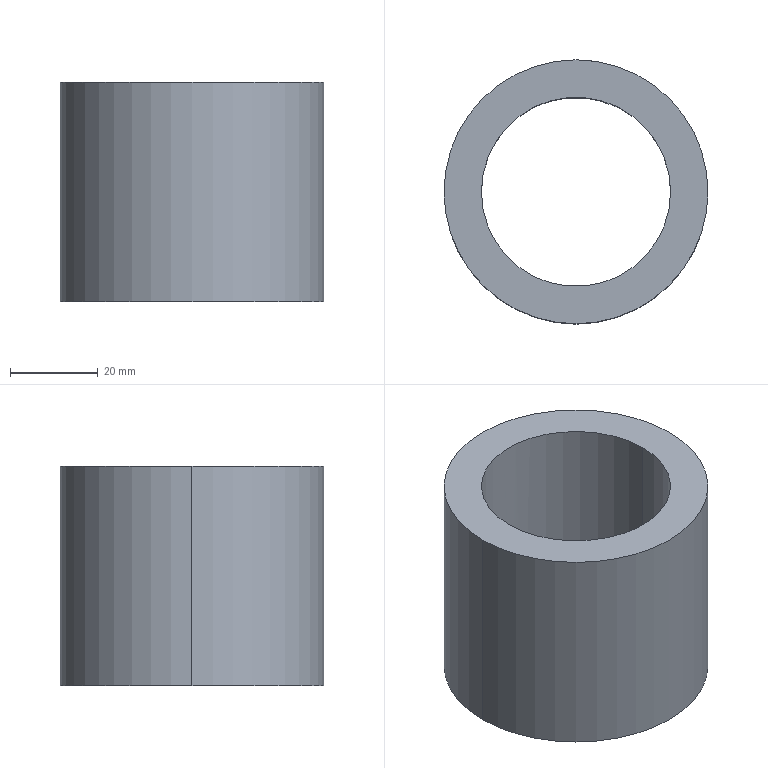Part | SolidWorks | features 3DProfileFeature 1, Cut 1, Extrusion 1, HoleWzd 1, ICE 1 | 1 solid | 8 faces | box 60 x 60 x 50 mm | volume 68595 mm3 | cylinder 6 | plane 2 | commonest cylinder face diameters 5 x2 43 x2 60 x2
STEP:
#1=CARTESIAN_POINT('',(4.954,20.921,-40.));
#2=VERTEX_POINT('',#1);
#3=CARTESIAN_POINT('',(-0.01248,21.5,-40.));
#4=VERTEX_POINT('',#3);
#5=CARTESIAN_POINT('',(4.954,20.921,-40.));
#6=CARTESIAN_POINT('',(4.954,20.921,-40.163));
#7=CARTESIAN_POINT('',(4.938,20.925,-40.325));
#8=CARTESIAN_POINT('',(4.876,20.94,-40.648));
#9=CARTESIAN_POINT('',(4.829,20.951,-40.806));
#10=CARTESIAN_POINT('',(4.706,20.979,-41.107));
#11=CARTESIAN_POINT('',(4.63,20.996,-41.252));
#12=CARTESIAN_POINT('',(4.451,21.034,-41.525));
#13=CARTESIAN_POINT('',(4.35,21.056,-41.651));
#14=CARTESIAN_POINT('',(4.123,21.101,-41.882));
#15=CARTESIAN_POINT('',(3.996,21.126,-41.987));
#16=CARTESIAN_POINT('',(3.729,21.175,-42.169));
#17=CARTESIAN_POINT('',(3.587,21.199,-42.246));
#18=CARTESIAN_POINT('',(3.288,21.248,-42.372));
#19=CARTESIAN_POINT('',(3.131,21.271,-42.42));
#20=CARTESIAN_POINT('',(2.815,21.316,-42.484));
#21=CARTESIAN_POINT('',(2.654,21.336,-42.5));
#22=CARTESIAN_POINT('',(2.325,21.375,-42.5));
#23=CARTESIAN_POINT('',(2.164,21.391,-42.484));
#24=CARTESIAN_POINT('',(1.845,21.421,-42.421));
#25=CARTESIAN_POINT('',(1.687,21.434,-42.373));
#26=CARTESIAN_POINT('',(1.384,21.456,-42.247));
#27=CARTESIAN_POINT('',(1.241,21.465,-42.171));
#28=CARTESIAN_POINT('',(0.9689,21.479,-41.989));
#29=CARTESIAN_POINT('',(0.8401,21.484,-41.884));
#30=CARTESIAN_POINT('',(0.6089,21.492,-41.654));
#31=CARTESIAN_POINT('',(0.505,21.494,-41.528));
#32=CARTESIAN_POINT('',(0.3212,21.498,-41.255));
#33=CARTESIAN_POINT('',(0.2431,21.499,-41.11));
#34=CARTESIAN_POINT('',(0.05455,21.5,-40.659));
#35=CARTESIAN_POINT('',(-0.01248,21.5,-40.331));
#36=CARTESIAN_POINT('',(-0.01248,21.5,-40.));
#37=B_SPLINE_CURVE_WITH_KNOTS('',3,(#5,#6,#7,#8,#9,#10,#11,#12,#13,#14,#15,#16,#17,#18,#19,#20,#21,#22,#23,#24,#25,#26,#27,#28,#29,#30,#31,#32,#33,#34,#35,#36),.UNSPECIFIED.,.F.,.F.,(4,2,2,2,2,2,2,2,2,2,2,2,2,2,2,4),(0.007823,0.008312,0.0088,0.009289,0.009778,0.01027,0.01076,0.01124,0.01173,0.01222,0.01271,0.0132,0.01369,0.01418,0.01467,0.01564),.UNSPECIFIED.);
#38=EDGE_CURVE('',#2,#4,#37,.T.);
#39=ORIENTED_EDGE('',*,*,#38,.F.);
#40=CARTESIAN_POINT('',(5.942,29.406,-40.));
#41=VERTEX_POINT('',#40);
#42=CARTESIAN_POINT('',(5.954,29.509,-40.));
#43=DIRECTION('',(0.1157,0.9933,0.));
#44=VECTOR('',#43,1000.);
#45=LINE('',#42,#44);
#46=EDGE_CURVE('',#2,#41,#45,.T.);
#47=ORIENTED_EDGE('',*,*,#46,.T.);
#48=CARTESIAN_POINT('',(0.9758,29.984,-40.));
#49=VERTEX_POINT('',#48);
#50=CARTESIAN_POINT('',(5.942,29.406,-40.));
#51=CARTESIAN_POINT('',(5.942,29.406,-40.163));
#52=CARTESIAN_POINT('',(5.927,29.409,-40.325));
#53=CARTESIAN_POINT('',(5.864,29.421,-40.648));
#54=CARTESIAN_POINT('',(5.816,29.431,-40.806));
#55=CARTESIAN_POINT('',(5.694,29.455,-41.107));
#56=CARTESIAN_POINT('',(5.618,29.469,-41.252));
#57=CARTESIAN_POINT('',(5.438,29.503,-41.525));
#58=CARTESIAN_POINT('',(5.336,29.522,-41.651));
#59=CARTESIAN_POINT('',(5.109,29.562,-41.882));
#60=CARTESIAN_POINT('',(4.982,29.584,-41.987));
#61=CARTESIAN_POINT('',(4.713,29.628,-42.169));
#62=CARTESIAN_POINT('',(4.572,29.65,-42.246));
#63=CARTESIAN_POINT('',(4.272,29.695,-42.372));
#64=CARTESIAN_POINT('',(4.115,29.717,-42.42));
#65=CARTESIAN_POINT('',(3.798,29.759,-42.484));
#66=CARTESIAN_POINT('',(3.637,29.779,-42.5));
#67=CARTESIAN_POINT('',(3.309,29.817,-42.5));
#68=CARTESIAN_POINT('',(3.147,29.835,-42.484));
#69=CARTESIAN_POINT('',(2.829,29.867,-42.421));
#70=CARTESIAN_POINT('',(2.671,29.881,-42.373));
#71=CARTESIAN_POINT('',(2.369,29.907,-42.247));
#72=CARTESIAN_POINT('',(2.226,29.918,-42.171));
#73=CARTESIAN_POINT('',(1.954,29.937,-41.99));
#74=CARTESIAN_POINT('',(1.826,29.945,-41.884));
#75=CARTESIAN_POINT('',(1.595,29.958,-41.654));
#76=CARTESIAN_POINT('',(1.491,29.963,-41.528));
#77=CARTESIAN_POINT('',(1.308,29.972,-41.255));
#78=CARTESIAN_POINT('',(1.23,29.975,-41.11));
#79=CARTESIAN_POINT('',(1.042,29.982,-40.659));
#80=CARTESIAN_POINT('',(0.9758,29.984,-40.33));
#81=CARTESIAN_POINT('',(0.9758,29.984,-40.));
#82=B_SPLINE_CURVE_WITH_KNOTS('',3,(#50,#51,#52,#53,#54,#55,#56,#57,#58,#59,#60,#61,#62,#63,#64,#65,#66,#67,#68,#69,#70,#71,#72,#73,#74,#75,#76,#77,#78,#79,#80,#81),.UNSPECIFIED.,.F.,.F.,(4,2,2,2,2,2,2,2,2,2,2,2,2,2,2,4),(0.00782,0.008308,0.008797,0.009285,0.009774,0.01026,0.01075,0.01124,0.01173,0.01222,0.01271,0.01319,0.01368,0.01417,0.01466,0.01564),.UNSPECIFIED.);
#83=EDGE_CURVE('',#41,#49,#82,.T.);
#84=ORIENTED_EDGE('',*,*,#83,.T.);
#85=CARTESIAN_POINT('',(0.9879,30.088,-40.));
#86=DIRECTION('',(0.1157,0.9933,0.));
#87=VECTOR('',#86,1000.);
#88=LINE('',#85,#87);
#89=EDGE_CURVE('',#4,#49,#88,.T.);
#90=ORIENTED_EDGE('',*,*,#89,.F.);
#91=EDGE_LOOP('',(#39,#47,#84,#90));
#92=FACE_OUTER_BOUND('',#91,.T.);
#93=CARTESIAN_POINT('',(3.471,29.799,-40.));
#94=DIRECTION('',(0.1157,0.9933,0.));
#95=DIRECTION('',(-0.9933,0.1157,0.));
#96=AXIS2_PLACEMENT_3D('',#93,#94,#95);
#97=CYLINDRICAL_SURFACE('',#96,2.5);
#98=ADVANCED_FACE('',(#92),#97,.F.);
#99=CARTESIAN_POINT('',(0.9758,29.984,-40.));
#100=CARTESIAN_POINT('',(0.9758,29.984,-39.835));
#101=CARTESIAN_POINT('',(0.9921,29.984,-39.672));
#102=CARTESIAN_POINT('',(1.056,29.981,-39.353));
#103=CARTESIAN_POINT('',(1.104,29.98,-39.194));
#104=CARTESIAN_POINT('',(1.23,29.975,-38.891));
#105=CARTESIAN_POINT('',(1.307,29.972,-38.747));
#106=CARTESIAN_POINT('',(1.489,29.963,-38.476));
#107=CARTESIAN_POINT('',(1.594,29.958,-38.347));
#108=CARTESIAN_POINT('',(1.825,29.945,-38.117));
#109=CARTESIAN_POINT('',(1.951,29.937,-38.013));
#110=CARTESIAN_POINT('',(2.223,29.918,-37.83));
#111=CARTESIAN_POINT('',(2.369,29.907,-37.753));
#112=CARTESIAN_POINT('',(2.669,29.881,-37.628));
#113=CARTESIAN_POINT('',(2.826,29.867,-37.58));
#114=CARTESIAN_POINT('',(3.147,29.835,-37.516));
#115=CARTESIAN_POINT('',(3.308,29.817,-37.5));
#116=CARTESIAN_POINT('',(3.632,29.78,-37.5));
#117=CARTESIAN_POINT('',(3.797,29.759,-37.516));
#118=CARTESIAN_POINT('',(4.115,29.717,-37.58));
#119=CARTESIAN_POINT('',(4.269,29.695,-37.627));
#120=CARTESIAN_POINT('',(4.569,29.65,-37.753));
#121=CARTESIAN_POINT('',(4.713,29.628,-37.831));
#122=CARTESIAN_POINT('',(4.981,29.584,-38.012));
#123=CARTESIAN_POINT('',(5.105,29.563,-38.115));
#124=CARTESIAN_POINT('',(5.336,29.522,-38.349));
#125=CARTESIAN_POINT('',(5.438,29.503,-38.475));
#126=CARTESIAN_POINT('',(5.616,29.47,-38.746));
#127=CARTESIAN_POINT('',(5.693,29.455,-38.892));
#128=CARTESIAN_POINT('',(5.817,29.431,-39.195));
#129=CARTESIAN_POINT('',(5.863,29.421,-39.351));
#130=CARTESIAN_POINT('',(5.926,29.409,-39.671));
#131=CARTESIAN_POINT('',(5.942,29.406,-39.837));
#132=CARTESIAN_POINT('',(5.942,29.406,-40.));
#133=B_SPLINE_CURVE_WITH_KNOTS('',3,(#99,#100,#101,#102,#103,#104,#105,#106,#107,#108,#109,#110,#111,#112,#113,#114,#115,#116,#117,#118,#119,#120,#121,#122,#123,#124,#125,#126,#127,#128,#129,#130,#131,#132),.UNSPECIFIED.,.F.,.F.,(4,2,2,2,2,2,2,2,2,2,2,2,2,2,2,2,4),(0.,0.0004887,0.0009774,0.001466,0.001955,0.002444,0.002932,0.003421,0.00391,0.004398,0.004887,0.005376,0.005865,0.006353,0.006842,0.007331,0.00782),.UNSPECIFIED.);
#134=EDGE_CURVE('',#49,#41,#133,.T.);
#135=ORIENTED_EDGE('',*,*,#134,.F.);
#136=ORIENTED_EDGE('',*,*,#83,.F.);
#137=EDGE_LOOP('',(#135,#136));
#138=FACE_BOUND('',#137,.T.);
#139=CARTESIAN_POINT('',(30.,0.,-50.));
#140=VERTEX_POINT('',#139);
#141=CARTESIAN_POINT('',(-30.,0.,-50.));
#142=VERTEX_POINT('',#141);
#143=CARTESIAN_POINT('',(0.,0.,-50.));
#144=DIRECTION('',(0.,0.,1.));
#145=DIRECTION('',(1.,0.,0.));
#146=AXIS2_PLACEMENT_3D('',#143,#144,#145);
#147=CIRCLE('',#146,30.);
#148=EDGE_CURVE('',#140,#142,#147,.T.);
#149=ORIENTED_EDGE('',*,*,#148,.T.);
#150=CARTESIAN_POINT('',(-30.,0.,0.));
#151=VERTEX_POINT('',#150);
#152=CARTESIAN_POINT('',(-30.,0.,-50.));
#153=DIRECTION('',(0.,0.,1.));
#154=VECTOR('',#153,1000.);
#155=LINE('',#152,#154);
#156=EDGE_CURVE('',#142,#151,#155,.T.);
#157=ORIENTED_EDGE('',*,*,#156,.T.);
#158=CARTESIAN_POINT('',(30.,0.,0.));
#159=VERTEX_POINT('',#158);
#160=CARTESIAN_POINT('',(0.,0.,0.));
#161=DIRECTION('',(0.,0.,1.));
#162=DIRECTION('',(1.,0.,0.));
#163=AXIS2_PLACEMENT_3D('',#160,#161,#162);
#164=CIRCLE('',#163,30.);
#165=EDGE_CURVE('',#159,#151,#164,.T.);
#166=ORIENTED_EDGE('',*,*,#165,.F.);
#167=CARTESIAN_POINT('',(30.,0.,-50.));
#168=DIRECTION('',(0.,0.,1.));
#169=VECTOR('',#168,1000.);
#170=LINE('',#167,#169);
#171=EDGE_CURVE('',#140,#159,#170,.T.);
#172=ORIENTED_EDGE('',*,*,#171,.F.);
#173=EDGE_LOOP('',(#149,#157,#166,#172));
#174=FACE_OUTER_BOUND('',#173,.T.);
#175=CARTESIAN_POINT('',(0.,0.,-50.));
#176=DIRECTION('',(0.,0.,1.));
#177=DIRECTION('',(1.,0.,0.));
#178=AXIS2_PLACEMENT_3D('',#175,#176,#177);
#179=CYLINDRICAL_SURFACE('',#178,30.);
#180=ADVANCED_FACE('',(#138,#174),#179,.T.);
#181=CARTESIAN_POINT('',(-21.5,0.,-50.));
#182=VERTEX_POINT('',#181);
#183=CARTESIAN_POINT('',(21.5,0.,-50.));
#184=VERTEX_POINT('',#183);
#185=CARTESIAN_POINT('',(0.,0.,-50.));
#186=DIRECTION('',(0.,0.,1.));
#187=DIRECTION('',(1.,0.,0.));
#188=AXIS2_PLACEMENT_3D('',#185,#186,#187);
#189=CIRCLE('',#188,21.5);
#190=EDGE_CURVE('',#182,#184,#189,.T.);
#191=ORIENTED_EDGE('',*,*,#190,.F.);
#192=CARTESIAN_POINT('',(-21.5,0.,0.));
#193=VERTEX_POINT('',#192);
#194=CARTESIAN_POINT('',(-21.5,0.,-50.));
#195=DIRECTION('',(0.,0.,1.));
#196=VECTOR('',#195,1000.);
#197=LINE('',#194,#196);
#198=EDGE_CURVE('',#182,#193,#197,.T.);
#199=ORIENTED_EDGE('',*,*,#198,.T.);
#200=CARTESIAN_POINT('',(21.5,0.,0.));
#201=VERTEX_POINT('',#200);
#202=CARTESIAN_POINT('',(0.,0.,0.));
#203=DIRECTION('',(0.,0.,1.));
#204=DIRECTION('',(1.,0.,0.));
#205=AXIS2_PLACEMENT_3D('',#202,#203,#204);
#206=CIRCLE('',#205,21.5);
#207=EDGE_CURVE('',#193,#201,#206,.T.);
#208=ORIENTED_EDGE('',*,*,#207,.T.);
#209=CARTESIAN_POINT('',(21.5,0.,-50.));
#210=DIRECTION('',(0.,0.,1.));
#211=VECTOR('',#210,1000.);
#212=LINE('',#209,#211);
#213=EDGE_CURVE('',#184,#201,#212,.T.);
#214=ORIENTED_EDGE('',*,*,#213,.F.);
#215=EDGE_LOOP('',(#191,#199,#208,#214));
#216=FACE_OUTER_BOUND('',#215,.T.);
#217=CARTESIAN_POINT('',(0.,0.,-50.));
#218=DIRECTION('',(0.,0.,1.));
#219=DIRECTION('',(1.,0.,0.));
#220=AXIS2_PLACEMENT_3D('',#217,#218,#219);
#221=CYLINDRICAL_SURFACE('',#220,21.5);
#222=ADVANCED_FACE('',(#216),#221,.F.);
#223=ORIENTED_EDGE('',*,*,#198,.F.);
#224=CARTESIAN_POINT('',(0.,0.,-50.));
#225=DIRECTION('',(0.,0.,1.));
#226=DIRECTION('',(1.,0.,0.));
#227=AXIS2_PLACEMENT_3D('',#224,#225,#226);
#228=CIRCLE('',#227,21.5);
#229=EDGE_CURVE('',#184,#182,#228,.T.);
#230=ORIENTED_EDGE('',*,*,#229,.F.);
#231=ORIENTED_EDGE('',*,*,#213,.T.);
#232=CARTESIAN_POINT('',(0.,0.,0.));
#233=DIRECTION('',(0.,0.,1.));
#234=DIRECTION('',(1.,0.,0.));
#235=AXIS2_PLACEMENT_3D('',#232,#233,#234);
#236=CIRCLE('',#235,21.5);
#237=EDGE_CURVE('',#201,#193,#236,.T.);
#238=ORIENTED_EDGE('',*,*,#237,.T.);
#239=EDGE_LOOP('',(#223,#230,#231,#238));
#240=FACE_OUTER_BOUND('',#239,.T.);
#241=CARTESIAN_POINT('',(-0.01248,21.5,-40.));
#242=CARTESIAN_POINT('',(-0.01248,21.5,-39.835));
#243=CARTESIAN_POINT('',(0.003868,21.5,-39.672));
#244=CARTESIAN_POINT('',(0.06789,21.5,-39.352));
#245=CARTESIAN_POINT('',(0.1163,21.5,-39.194));
#246=CARTESIAN_POINT('',(0.2426,21.499,-38.891));
#247=CARTESIAN_POINT('',(0.3199,21.498,-38.747));
#248=CARTESIAN_POINT('',(0.5021,21.494,-38.476));
#249=CARTESIAN_POINT('',(0.6081,21.492,-38.347));
#250=CARTESIAN_POINT('',(0.8392,21.484,-38.117));
#251=CARTESIAN_POINT('',(0.9652,21.479,-38.013));
#252=CARTESIAN_POINT('',(1.239,21.465,-37.83));
#253=CARTESIAN_POINT('',(1.384,21.456,-37.753));
#254=CARTESIAN_POINT('',(1.684,21.434,-37.628));
#255=CARTESIAN_POINT('',(1.842,21.422,-37.58));
#256=CARTESIAN_POINT('',(2.163,21.392,-37.516));
#257=CARTESIAN_POINT('',(2.325,21.375,-37.5));
#258=CARTESIAN_POINT('',(2.649,21.337,-37.5));
#259=CARTESIAN_POINT('',(2.813,21.316,-37.516));
#260=CARTESIAN_POINT('',(3.131,21.271,-37.58));
#261=CARTESIAN_POINT('',(3.285,21.248,-37.627));
#262=CARTESIAN_POINT('',(3.585,21.2,-37.753));
#263=CARTESIAN_POINT('',(3.729,21.175,-37.831));
#264=CARTESIAN_POINT('',(3.996,21.126,-38.012));
#265=CARTESIAN_POINT('',(4.12,21.102,-38.115));
#266=CARTESIAN_POINT('',(4.35,21.056,-38.349));
#267=CARTESIAN_POINT('',(4.451,21.034,-38.475));
#268=CARTESIAN_POINT('',(4.629,20.996,-38.745));
#269=CARTESIAN_POINT('',(4.706,20.979,-38.892));
#270=CARTESIAN_POINT('',(4.829,20.951,-39.194));
#271=CARTESIAN_POINT('',(4.875,20.94,-39.35));
#272=CARTESIAN_POINT('',(4.938,20.925,-39.671));
#273=CARTESIAN_POINT('',(4.954,20.921,-39.837));
#274=CARTESIAN_POINT('',(4.954,20.921,-40.));
#275=B_SPLINE_CURVE_WITH_KNOTS('',3,(#241,#242,#243,#244,#245,#246,#247,#248,#249,#250,#251,#252,#253,#254,#255,#256,#257,#258,#259,#260,#261,#262,#263,#264,#265,#266,#267,#268,#269,#270,#271,#272,#273,#274),.UNSPECIFIED.,.F.,.F.,(4,2,2,2,2,2,2,2,2,2,2,2,2,2,2,2,4),(0.,0.0004889,0.0009778,0.001467,0.001956,0.002445,0.002934,0.003422,0.003911,0.0044,0.004889,0.005378,0.005867,0.006356,0.006845,0.007334,0.007823),.UNSPECIFIED.);
#276=EDGE_CURVE('',#4,#2,#275,.T.);
#277=ORIENTED_EDGE('',*,*,#276,.T.);
#278=ORIENTED_EDGE('',*,*,#38,.T.);
#279=EDGE_LOOP('',(#277,#278));
#280=FACE_BOUND('',#279,.T.);
#281=CARTESIAN_POINT('',(0.,0.,-50.));
#282=DIRECTION('',(0.,0.,1.));
#283=DIRECTION('',(1.,0.,0.));
#284=AXIS2_PLACEMENT_3D('',#281,#282,#283);
#285=CYLINDRICAL_SURFACE('',#284,21.5);
#286=ADVANCED_FACE('',(#240,#280),#285,.F.);
#287=ORIENTED_EDGE('',*,*,#165,.T.);
#288=CARTESIAN_POINT('',(0.,0.,0.));
#289=DIRECTION('',(0.,0.,1.));
#290=DIRECTION('',(1.,0.,0.));
#291=AXIS2_PLACEMENT_3D('',#288,#289,#290);
#292=CIRCLE('',#291,30.);
#293=EDGE_CURVE('',#151,#159,#292,.T.);
#294=ORIENTED_EDGE('',*,*,#293,.T.);
#295=EDGE_LOOP('',(#287,#294));
#296=FACE_OUTER_BOUND('',#295,.T.);
#297=ORIENTED_EDGE('',*,*,#237,.F.);
#298=ORIENTED_EDGE('',*,*,#207,.F.);
#299=EDGE_LOOP('',(#297,#298));
#300=FACE_BOUND('',#299,.T.);
#301=CARTESIAN_POINT('',(0.,0.,0.));
#302=DIRECTION('',(0.,0.,1.));
#303=DIRECTION('',(1.,0.,0.));
#304=AXIS2_PLACEMENT_3D('',#301,#302,#303);
#305=PLANE('',#304);
#306=ADVANCED_FACE('',(#296,#300),#305,.T.);
#307=ORIENTED_EDGE('',*,*,#156,.F.);
#308=CARTESIAN_POINT('',(0.,0.,-50.));
#309=DIRECTION('',(0.,0.,1.));
#310=DIRECTION('',(1.,0.,0.));
#311=AXIS2_PLACEMENT_3D('',#308,#309,#310);
#312=CIRCLE('',#311,30.);
#313=EDGE_CURVE('',#142,#140,#312,.T.);
#314=ORIENTED_EDGE('',*,*,#313,.T.);
#315=ORIENTED_EDGE('',*,*,#171,.T.);
#316=ORIENTED_EDGE('',*,*,#293,.F.);
#317=EDGE_LOOP('',(#307,#314,#315,#316));
#318=FACE_OUTER_BOUND('',#317,.T.);
#319=CARTESIAN_POINT('',(0.,0.,-50.));
#320=DIRECTION('',(0.,0.,1.));
#321=DIRECTION('',(1.,0.,0.));
#322=AXIS2_PLACEMENT_3D('',#319,#320,#321);
#323=CYLINDRICAL_SURFACE('',#322,30.);
#324=ADVANCED_FACE('',(#318),#323,.T.);
#325=ORIENTED_EDGE('',*,*,#229,.T.);
#326=ORIENTED_EDGE('',*,*,#190,.T.);
#327=EDGE_LOOP('',(#325,#326));
#328=FACE_BOUND('',#327,.T.);
#329=ORIENTED_EDGE('',*,*,#148,.F.);
#330=ORIENTED_EDGE('',*,*,#313,.F.);
#331=EDGE_LOOP('',(#329,#330));
#332=FACE_OUTER_BOUND('',#331,.T.);
#333=CARTESIAN_POINT('',(0.,0.,-50.));
#334=DIRECTION('',(0.,0.,1.));
#335=DIRECTION('',(1.,0.,0.));
#336=AXIS2_PLACEMENT_3D('',#333,#334,#335);
#337=PLANE('',#336);
#338=ADVANCED_FACE('',(#328,#332),#337,.F.);
#339=ORIENTED_EDGE('',*,*,#46,.F.);
#340=ORIENTED_EDGE('',*,*,#276,.F.);
#341=ORIENTED_EDGE('',*,*,#89,.T.);
#342=ORIENTED_EDGE('',*,*,#134,.T.);
#343=EDGE_LOOP('',(#339,#340,#341,#342));
#344=FACE_OUTER_BOUND('',#343,.T.);
#345=CARTESIAN_POINT('',(3.471,29.799,-40.));
#346=DIRECTION('',(0.1157,0.9933,0.));
#347=DIRECTION('',(-0.9933,0.1157,0.));
#348=AXIS2_PLACEMENT_3D('',#345,#346,#347);
#349=CYLINDRICAL_SURFACE('',#348,2.5);
#350=ADVANCED_FACE('',(#344),#349,.F.);
#351=CLOSED_SHELL('',(#98,#180,#222,#286,#306,#324,#338,#350));
#352=MANIFOLD_SOLID_BREP('',#351);
#353=CARTESIAN_POINT('',(0.,0.,0.));
#354=DIRECTION('',(0.,0.,1.));
#355=DIRECTION('',(1.,0.,0.));
#356=AXIS2_PLACEMENT_3D('',#353,#354,#355);
#357=(LENGTH_UNIT()NAMED_UNIT(*)SI_UNIT(.MILLI.,.METRE.));
#358=UNCERTAINTY_MEASURE_WITH_UNIT(LENGTH_MEASURE(0.00001),#357,'','');
#359=(NAMED_UNIT(*)PLANE_ANGLE_UNIT()SI_UNIT($,.RADIAN.));
#360=(NAMED_UNIT(*)SI_UNIT($,.STERADIAN.)SOLID_ANGLE_UNIT());
#361=(GEOMETRIC_REPRESENTATION_CONTEXT(3)GLOBAL_UNCERTAINTY_ASSIGNED_CONTEXT((#358))GLOBAL_UNIT_ASSIGNED_CONTEXT((#357,#359,#360))REPRESENTATION_CONTEXT('',''));
#362=ADVANCED_BREP_SHAPE_REPRESENTATION('',(#352,#356),#361);